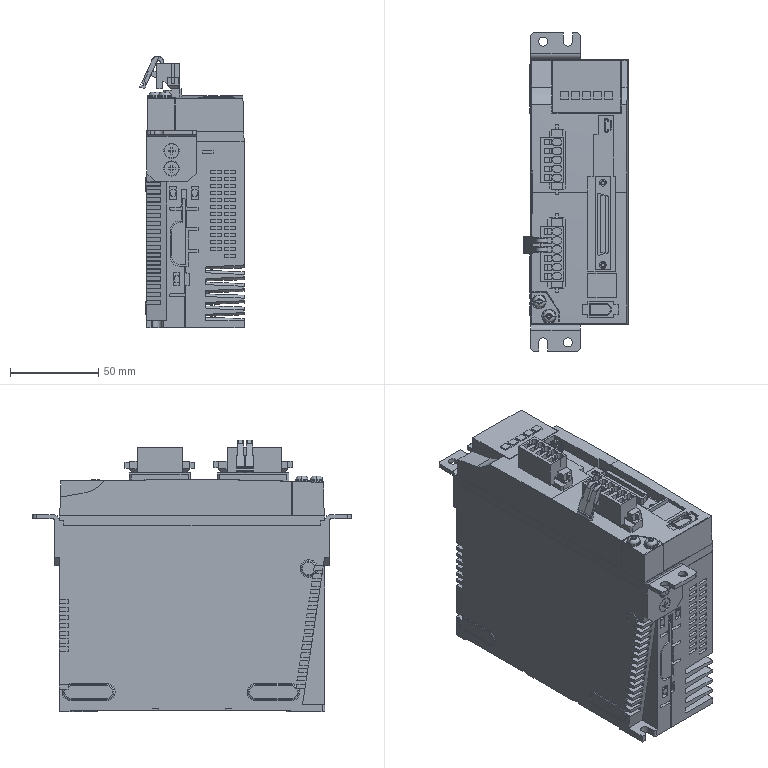Part | STEP file | MBDLN25SE | 1 solid | 1620 faces | box 58.866 x 180 x 153.541 mm | volume 995298 mm3 | plane 1079 | cylinder 469 | cone 49 | torus 23 | commonest cylinder face diameters 0.4 x90 2 x85 1 x56 1.4 x50 3 x48 0.6 x34